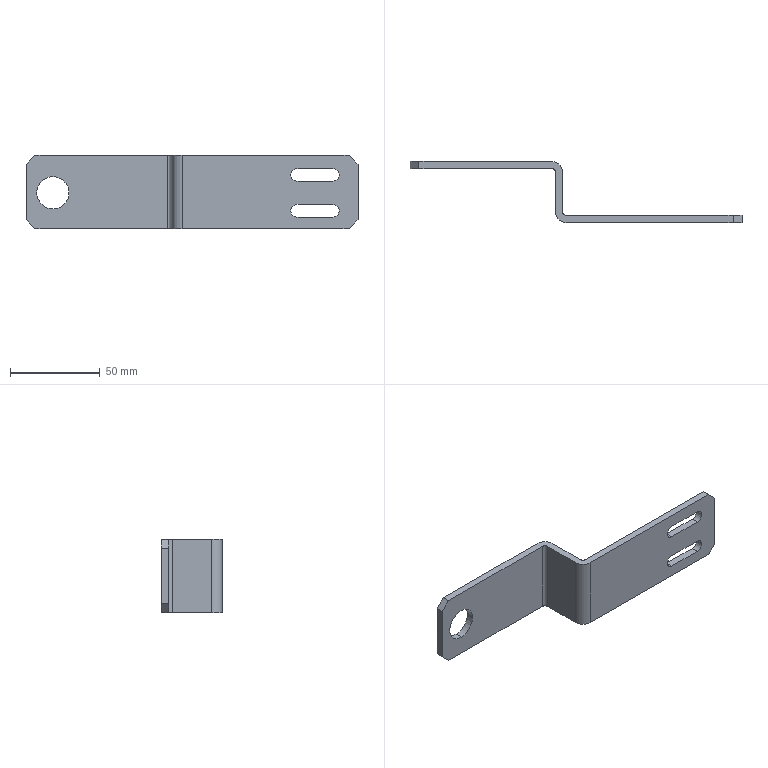Part | SolidWorks | features ICE 4, Fillet 2, Chamfer 1, Extrusion 1, HoleWzd 1 | 1 solid | 28 faces | box 185 x 34 x 40.884 mm | volume 31953 mm3 | plane 18 | cylinder 10 | commonest cylinder face diameters 7 x4 4 x2 12 x2 18 x2
STEP:
#1=CARTESIAN_POINT('',(15.,4.,29.));
#2=VERTEX_POINT('',#1);
#3=CARTESIAN_POINT('',(15.,4.,11.));
#4=VERTEX_POINT('',#3);
#5=CARTESIAN_POINT('',(15.,4.,20.));
#6=DIRECTION('',(0.,-1.,0.));
#7=DIRECTION('',(0.,0.,-1.));
#8=AXIS2_PLACEMENT_3D('',#5,#6,#7);
#9=CIRCLE('',#8,9.);
#10=EDGE_CURVE('',#2,#4,#9,.T.);
#11=ORIENTED_EDGE('',*,*,#10,.F.);
#12=CARTESIAN_POINT('',(15.,0.,29.));
#13=VERTEX_POINT('',#12);
#14=CARTESIAN_POINT('',(15.,0.,29.));
#15=DIRECTION('',(0.,-1.,0.));
#16=VECTOR('',#15,1000.);
#17=LINE('',#14,#16);
#18=EDGE_CURVE('',#2,#13,#17,.T.);
#19=ORIENTED_EDGE('',*,*,#18,.T.);
#20=CARTESIAN_POINT('',(15.,0.,11.));
#21=VERTEX_POINT('',#20);
#22=CARTESIAN_POINT('',(15.,0.,20.));
#23=DIRECTION('',(0.,-1.,0.));
#24=DIRECTION('',(0.,0.,-1.));
#25=AXIS2_PLACEMENT_3D('',#22,#23,#24);
#26=CIRCLE('',#25,9.);
#27=EDGE_CURVE('',#13,#21,#26,.T.);
#28=ORIENTED_EDGE('',*,*,#27,.T.);
#29=CARTESIAN_POINT('',(15.,0.,11.));
#30=DIRECTION('',(0.,-1.,0.));
#31=VECTOR('',#30,1000.);
#32=LINE('',#29,#31);
#33=EDGE_CURVE('',#4,#21,#32,.T.);
#34=ORIENTED_EDGE('',*,*,#33,.F.);
#35=EDGE_LOOP('',(#11,#19,#28,#34));
#36=FACE_OUTER_BOUND('',#35,.T.);
#37=CARTESIAN_POINT('',(15.,0.,20.));
#38=DIRECTION('',(0.,-1.,0.));
#39=DIRECTION('',(0.,0.,-1.));
#40=AXIS2_PLACEMENT_3D('',#37,#38,#39);
#41=CYLINDRICAL_SURFACE('',#40,9.);
#42=ADVANCED_FACE('',(#36),#41,.F.);
#43=CARTESIAN_POINT('',(0.,0.,35.884));
#44=VERTEX_POINT('',#43);
#45=CARTESIAN_POINT('',(0.,0.,5.));
#46=VERTEX_POINT('',#45);
#47=CARTESIAN_POINT('',(0.,0.,40.884));
#48=DIRECTION('',(0.,0.,-1.));
#49=VECTOR('',#48,1000.);
#50=LINE('',#47,#49);
#51=EDGE_CURVE('',#44,#46,#50,.T.);
#52=ORIENTED_EDGE('',*,*,#51,.F.);
#53=CARTESIAN_POINT('',(0.,4.,35.884));
#54=VERTEX_POINT('',#53);
#55=CARTESIAN_POINT('',(0.,4.,35.884));
#56=DIRECTION('',(0.,1.,0.));
#57=VECTOR('',#56,1000.);
#58=LINE('',#55,#57);
#59=EDGE_CURVE('',#44,#54,#58,.T.);
#60=ORIENTED_EDGE('',*,*,#59,.T.);
#61=CARTESIAN_POINT('',(0.,4.,5.));
#62=VERTEX_POINT('',#61);
#63=CARTESIAN_POINT('',(0.,4.,40.884));
#64=DIRECTION('',(0.,0.,-1.));
#65=VECTOR('',#64,1000.);
#66=LINE('',#63,#65);
#67=EDGE_CURVE('',#54,#62,#66,.T.);
#68=ORIENTED_EDGE('',*,*,#67,.T.);
#69=CARTESIAN_POINT('',(0.,4.,5.));
#70=DIRECTION('',(0.,-1.,0.));
#71=VECTOR('',#70,1000.);
#72=LINE('',#69,#71);
#73=EDGE_CURVE('',#62,#46,#72,.T.);
#74=ORIENTED_EDGE('',*,*,#73,.T.);
#75=EDGE_LOOP('',(#52,#60,#68,#74));
#76=FACE_OUTER_BOUND('',#75,.T.);
#77=CARTESIAN_POINT('',(0.,4.,40.884));
#78=DIRECTION('',(-1.,0.,0.));
#79=DIRECTION('',(0.,0.,1.));
#80=AXIS2_PLACEMENT_3D('',#77,#78,#79);
#81=PLANE('',#80);
#82=ADVANCED_FACE('',(#76),#81,.T.);
#83=CARTESIAN_POINT('',(81.,-2.,40.884));
#84=VERTEX_POINT('',#83);
#85=CARTESIAN_POINT('',(81.,-24.,40.884));
#86=VERTEX_POINT('',#85);
#87=CARTESIAN_POINT('',(81.,0.,40.884));
#88=DIRECTION('',(0.,-1.,0.));
#89=VECTOR('',#88,1000.);
#90=LINE('',#87,#89);
#91=EDGE_CURVE('',#84,#86,#90,.T.);
#92=ORIENTED_EDGE('',*,*,#91,.T.);
#93=CARTESIAN_POINT('',(87.,-30.,40.884));
#94=VERTEX_POINT('',#93);
#95=CARTESIAN_POINT('',(87.,-24.,40.884));
#96=DIRECTION('',(0.,0.,1.));
#97=DIRECTION('',(1.,0.,0.));
#98=AXIS2_PLACEMENT_3D('',#95,#96,#97);
#99=CIRCLE('',#98,6.);
#100=EDGE_CURVE('',#86,#94,#99,.T.);
#101=ORIENTED_EDGE('',*,*,#100,.T.);
#102=CARTESIAN_POINT('',(180.,-30.,40.884));
#103=VERTEX_POINT('',#102);
#104=CARTESIAN_POINT('',(185.,-30.,40.884));
#105=DIRECTION('',(-1.,0.,0.));
#106=VECTOR('',#105,1000.);
#107=LINE('',#104,#106);
#108=EDGE_CURVE('',#103,#94,#107,.T.);
#109=ORIENTED_EDGE('',*,*,#108,.F.);
#110=CARTESIAN_POINT('',(180.,-26.,40.884));
#111=VERTEX_POINT('',#110);
#112=CARTESIAN_POINT('',(180.,4.,40.884));
#113=DIRECTION('',(0.,1.,0.));
#114=VECTOR('',#113,1000.);
#115=LINE('',#112,#114);
#116=EDGE_CURVE('',#103,#111,#115,.T.);
#117=ORIENTED_EDGE('',*,*,#116,.T.);
#118=CARTESIAN_POINT('',(87.,-26.,40.884));
#119=VERTEX_POINT('',#118);
#120=CARTESIAN_POINT('',(185.,-26.,40.884));
#121=DIRECTION('',(-1.,0.,0.));
#122=VECTOR('',#121,1000.);
#123=LINE('',#120,#122);
#124=EDGE_CURVE('',#111,#119,#123,.T.);
#125=ORIENTED_EDGE('',*,*,#124,.T.);
#126=CARTESIAN_POINT('',(85.,-24.,40.884));
#127=VERTEX_POINT('',#126);
#128=CARTESIAN_POINT('',(87.,-24.,40.884));
#129=DIRECTION('',(0.,0.,-1.));
#130=DIRECTION('',(1.,0.,0.));
#131=AXIS2_PLACEMENT_3D('',#128,#129,#130);
#132=CIRCLE('',#131,2.);
#133=EDGE_CURVE('',#119,#127,#132,.T.);
#134=ORIENTED_EDGE('',*,*,#133,.T.);
#135=CARTESIAN_POINT('',(85.,-2.,40.884));
#136=VERTEX_POINT('',#135);
#137=CARTESIAN_POINT('',(85.,-26.,40.884));
#138=DIRECTION('',(0.,1.,0.));
#139=VECTOR('',#138,1000.);
#140=LINE('',#137,#139);
#141=EDGE_CURVE('',#127,#136,#140,.T.);
#142=ORIENTED_EDGE('',*,*,#141,.T.);
#143=CARTESIAN_POINT('',(79.,4.,40.884));
#144=VERTEX_POINT('',#143);
#145=CARTESIAN_POINT('',(79.,-2.,40.884));
#146=DIRECTION('',(0.,0.,1.));
#147=DIRECTION('',(1.,0.,0.));
#148=AXIS2_PLACEMENT_3D('',#145,#146,#147);
#149=CIRCLE('',#148,6.);
#150=EDGE_CURVE('',#136,#144,#149,.T.);
#151=ORIENTED_EDGE('',*,*,#150,.T.);
#152=CARTESIAN_POINT('',(5.,4.,40.884));
#153=VERTEX_POINT('',#152);
#154=CARTESIAN_POINT('',(185.,4.,40.884));
#155=DIRECTION('',(-1.,0.,0.));
#156=VECTOR('',#155,1000.);
#157=LINE('',#154,#156);
#158=EDGE_CURVE('',#144,#153,#157,.T.);
#159=ORIENTED_EDGE('',*,*,#158,.T.);
#160=CARTESIAN_POINT('',(5.,0.,40.884));
#161=VERTEX_POINT('',#160);
#162=CARTESIAN_POINT('',(5.,4.,40.884));
#163=DIRECTION('',(0.,-1.,0.));
#164=VECTOR('',#163,1000.);
#165=LINE('',#162,#164);
#166=EDGE_CURVE('',#153,#161,#165,.T.);
#167=ORIENTED_EDGE('',*,*,#166,.T.);
#168=CARTESIAN_POINT('',(79.,0.,40.884));
#169=VERTEX_POINT('',#168);
#170=CARTESIAN_POINT('',(0.,0.,40.884));
#171=DIRECTION('',(1.,0.,0.));
#172=VECTOR('',#171,1000.);
#173=LINE('',#170,#172);
#174=EDGE_CURVE('',#161,#169,#173,.T.);
#175=ORIENTED_EDGE('',*,*,#174,.T.);
#176=CARTESIAN_POINT('',(79.,-2.,40.884));
#177=DIRECTION('',(0.,0.,-1.));
#178=DIRECTION('',(1.,0.,0.));
#179=AXIS2_PLACEMENT_3D('',#176,#177,#178);
#180=CIRCLE('',#179,2.);
#181=EDGE_CURVE('',#169,#84,#180,.T.);
#182=ORIENTED_EDGE('',*,*,#181,.T.);
#183=EDGE_LOOP('',(#92,#101,#109,#117,#125,#134,#142,#151,#159,#167,#175,#182));
#184=FACE_OUTER_BOUND('',#183,.T.);
#185=CARTESIAN_POINT('',(185.,4.,40.884));
#186=DIRECTION('',(0.,0.,1.));
#187=DIRECTION('',(1.,0.,0.));
#188=AXIS2_PLACEMENT_3D('',#185,#186,#187);
#189=PLANE('',#188);
#190=ADVANCED_FACE('',(#184),#189,.T.);
#191=CARTESIAN_POINT('',(185.,-30.,5.));
#192=VERTEX_POINT('',#191);
#193=CARTESIAN_POINT('',(185.,-30.,35.884));
#194=VERTEX_POINT('',#193);
#195=CARTESIAN_POINT('',(185.,-30.,0.));
#196=DIRECTION('',(0.,0.,1.));
#197=VECTOR('',#196,1000.);
#198=LINE('',#195,#197);
#199=EDGE_CURVE('',#192,#194,#198,.T.);
#200=ORIENTED_EDGE('',*,*,#199,.F.);
#201=CARTESIAN_POINT('',(185.,-26.,5.));
#202=VERTEX_POINT('',#201);
#203=CARTESIAN_POINT('',(185.,4.,5.));
#204=DIRECTION('',(0.,1.,0.));
#205=VECTOR('',#204,1000.);
#206=LINE('',#203,#205);
#207=EDGE_CURVE('',#192,#202,#206,.T.);
#208=ORIENTED_EDGE('',*,*,#207,.T.);
#209=CARTESIAN_POINT('',(185.,-26.,35.884));
#210=VERTEX_POINT('',#209);
#211=CARTESIAN_POINT('',(185.,-26.,40.884));
#212=DIRECTION('',(0.,0.,-1.));
#213=VECTOR('',#212,1000.);
#214=LINE('',#211,#213);
#215=EDGE_CURVE('',#210,#202,#214,.T.);
#216=ORIENTED_EDGE('',*,*,#215,.F.);
#217=CARTESIAN_POINT('',(185.,4.,35.884));
#218=DIRECTION('',(0.,-1.,0.));
#219=VECTOR('',#218,1000.);
#220=LINE('',#217,#219);
#221=EDGE_CURVE('',#210,#194,#220,.T.);
#222=ORIENTED_EDGE('',*,*,#221,.T.);
#223=EDGE_LOOP('',(#200,#208,#216,#222));
#224=FACE_OUTER_BOUND('',#223,.T.);
#225=CARTESIAN_POINT('',(185.,4.,0.));
#226=DIRECTION('',(1.,0.,0.));
#227=DIRECTION('',(0.,0.,-1.));
#228=AXIS2_PLACEMENT_3D('',#225,#226,#227);
#229=PLANE('',#228);
#230=ADVANCED_FACE('',(#224),#229,.T.);
#231=CARTESIAN_POINT('',(87.,-30.,0.));
#232=VERTEX_POINT('',#231);
#233=CARTESIAN_POINT('',(180.,-30.,0.));
#234=VERTEX_POINT('',#233);
#235=CARTESIAN_POINT('',(0.,-30.,0.));
#236=DIRECTION('',(1.,0.,0.));
#237=VECTOR('',#236,1000.);
#238=LINE('',#235,#237);
#239=EDGE_CURVE('',#232,#234,#238,.T.);
#240=ORIENTED_EDGE('',*,*,#239,.F.);
#241=CARTESIAN_POINT('',(81.,-24.,0.));
#242=VERTEX_POINT('',#241);
#243=CARTESIAN_POINT('',(87.,-24.,0.));
#244=DIRECTION('',(0.,0.,-1.));
#245=DIRECTION('',(-1.,0.,0.));
#246=AXIS2_PLACEMENT_3D('',#243,#244,#245);
#247=CIRCLE('',#246,6.);
#248=EDGE_CURVE('',#232,#242,#247,.T.);
#249=ORIENTED_EDGE('',*,*,#248,.T.);
#250=CARTESIAN_POINT('',(81.,-2.,0.));
#251=VERTEX_POINT('',#250);
#252=CARTESIAN_POINT('',(81.,0.,0.));
#253=DIRECTION('',(0.,-1.,0.));
#254=VECTOR('',#253,1000.);
#255=LINE('',#252,#254);
#256=EDGE_CURVE('',#251,#242,#255,.T.);
#257=ORIENTED_EDGE('',*,*,#256,.F.);
#258=CARTESIAN_POINT('',(79.,0.,0.));
#259=VERTEX_POINT('',#258);
#260=CARTESIAN_POINT('',(79.,-2.,0.));
#261=DIRECTION('',(0.,0.,1.));
#262=DIRECTION('',(-1.,0.,0.));
#263=AXIS2_PLACEMENT_3D('',#260,#261,#262);
#264=CIRCLE('',#263,2.);
#265=EDGE_CURVE('',#251,#259,#264,.T.);
#266=ORIENTED_EDGE('',*,*,#265,.T.);
#267=CARTESIAN_POINT('',(5.,0.,0.));
#268=VERTEX_POINT('',#267);
#269=CARTESIAN_POINT('',(0.,0.,0.));
#270=DIRECTION('',(1.,0.,0.));
#271=VECTOR('',#270,1000.);
#272=LINE('',#269,#271);
#273=EDGE_CURVE('',#268,#259,#272,.T.);
#274=ORIENTED_EDGE('',*,*,#273,.F.);
#275=CARTESIAN_POINT('',(5.,4.,0.));
#276=VERTEX_POINT('',#275);
#277=CARTESIAN_POINT('',(5.,4.,0.));
#278=DIRECTION('',(0.,1.,0.));
#279=VECTOR('',#278,1000.);
#280=LINE('',#277,#279);
#281=EDGE_CURVE('',#268,#276,#280,.T.);
#282=ORIENTED_EDGE('',*,*,#281,.T.);
#283=CARTESIAN_POINT('',(79.,4.,0.));
#284=VERTEX_POINT('',#283);
#285=CARTESIAN_POINT('',(0.,4.,0.));
#286=DIRECTION('',(1.,0.,0.));
#287=VECTOR('',#286,1000.);
#288=LINE('',#285,#287);
#289=EDGE_CURVE('',#276,#284,#288,.T.);
#290=ORIENTED_EDGE('',*,*,#289,.T.);
#291=CARTESIAN_POINT('',(85.,-2.,0.));
#292=VERTEX_POINT('',#291);
#293=CARTESIAN_POINT('',(79.,-2.,0.));
#294=DIRECTION('',(0.,0.,-1.));
#295=DIRECTION('',(-1.,0.,0.));
#296=AXIS2_PLACEMENT_3D('',#293,#294,#295);
#297=CIRCLE('',#296,6.);
#298=EDGE_CURVE('',#284,#292,#297,.T.);
#299=ORIENTED_EDGE('',*,*,#298,.T.);
#300=CARTESIAN_POINT('',(85.,-24.,0.));
#301=VERTEX_POINT('',#300);
#302=CARTESIAN_POINT('',(85.,-26.,0.));
#303=DIRECTION('',(0.,1.,0.));
#304=VECTOR('',#303,1000.);
#305=LINE('',#302,#304);
#306=EDGE_CURVE('',#301,#292,#305,.T.);
#307=ORIENTED_EDGE('',*,*,#306,.F.);
#308=CARTESIAN_POINT('',(87.,-26.,0.));
#309=VERTEX_POINT('',#308);
#310=CARTESIAN_POINT('',(87.,-24.,0.));
#311=DIRECTION('',(0.,0.,1.));
#312=DIRECTION('',(-1.,0.,0.));
#313=AXIS2_PLACEMENT_3D('',#310,#311,#312);
#314=CIRCLE('',#313,2.);
#315=EDGE_CURVE('',#301,#309,#314,.T.);
#316=ORIENTED_EDGE('',*,*,#315,.T.);
#317=CARTESIAN_POINT('',(180.,-26.,0.));
#318=VERTEX_POINT('',#317);
#319=CARTESIAN_POINT('',(185.,-26.,0.));
#320=DIRECTION('',(-1.,0.,0.));
#321=VECTOR('',#320,1000.);
#322=LINE('',#319,#321);
#323=EDGE_CURVE('',#318,#309,#322,.T.);
#324=ORIENTED_EDGE('',*,*,#323,.F.);
#325=CARTESIAN_POINT('',(180.,4.,0.));
#326=DIRECTION('',(0.,-1.,0.));
#327=VECTOR('',#326,1000.);
#328=LINE('',#325,#327);
#329=EDGE_CURVE('',#318,#234,#328,.T.);
#330=ORIENTED_EDGE('',*,*,#329,.T.);
#331=EDGE_LOOP('',(#240,#249,#257,#266,#274,#282,#290,#299,#307,#316,#324,#330));
#332=FACE_OUTER_BOUND('',#331,.T.);
#333=CARTESIAN_POINT('',(0.,4.,0.));
#334=DIRECTION('',(0.,0.,-1.));
#335=DIRECTION('',(-1.,0.,0.));
#336=AXIS2_PLACEMENT_3D('',#333,#334,#335);
#337=PLANE('',#336);
#338=ADVANCED_FACE('',(#332),#337,.T.);
#339=CARTESIAN_POINT('',(15.,4.,20.));
#340=DIRECTION('',(0.,-1.,0.));
#341=DIRECTION('',(0.,0.,-1.));
#342=AXIS2_PLACEMENT_3D('',#339,#340,#341);
#343=CIRCLE('',#342,9.);
#344=EDGE_CURVE('',#4,#2,#343,.T.);
#345=ORIENTED_EDGE('',*,*,#344,.T.);
#346=ORIENTED_EDGE('',*,*,#10,.T.);
#347=EDGE_LOOP('',(#345,#346));
#348=FACE_BOUND('',#347,.T.);
#349=ORIENTED_EDGE('',*,*,#158,.F.);
#350=CARTESIAN_POINT('',(79.,4.,0.));
#351=DIRECTION('',(0.,0.,-1.));
#352=VECTOR('',#351,1000.);
#353=LINE('',#350,#352);
#354=EDGE_CURVE('',#144,#284,#353,.T.);
#355=ORIENTED_EDGE('',*,*,#354,.T.);
#356=ORIENTED_EDGE('',*,*,#289,.F.);
#357=CARTESIAN_POINT('',(0.,4.,5.));
#358=DIRECTION('',(-0.7071,0.,0.7071));
#359=VECTOR('',#358,1000.);
#360=LINE('',#357,#359);
#361=EDGE_CURVE('',#276,#62,#360,.T.);
#362=ORIENTED_EDGE('',*,*,#361,.T.);
#363=ORIENTED_EDGE('',*,*,#67,.F.);
#364=CARTESIAN_POINT('',(5.,4.,40.884));
#365=DIRECTION('',(0.7071,0.,0.7071));
#366=VECTOR('',#365,1000.);
#367=LINE('',#364,#366);
#368=EDGE_CURVE('',#54,#153,#367,.T.);
#369=ORIENTED_EDGE('',*,*,#368,.T.);
#370=EDGE_LOOP('',(#349,#355,#356,#362,#363,#369));
#371=FACE_OUTER_BOUND('',#370,.T.);
#372=CARTESIAN_POINT('',(0.,4.,0.));
#373=DIRECTION('',(0.,-1.,0.));
#374=DIRECTION('',(0.,0.,-1.));
#375=AXIS2_PLACEMENT_3D('',#372,#373,#374);
#376=PLANE('',#375);
#377=ADVANCED_FACE('',(#348,#371),#376,.F.);
#378=CARTESIAN_POINT('',(151.,-30.,26.5));
#379=VERTEX_POINT('',#378);
#380=CARTESIAN_POINT('',(151.,-30.,33.5));
#381=VERTEX_POINT('',#380);
#382=CARTESIAN_POINT('',(151.,-30.,30.));
#383=DIRECTION('',(0.,1.,0.));
#384=DIRECTION('',(0.,0.,1.));
#385=AXIS2_PLACEMENT_3D('',#382,#383,#384);
#386=CIRCLE('',#385,3.5);
#387=EDGE_CURVE('',#379,#381,#386,.T.);
#388=ORIENTED_EDGE('',*,*,#387,.T.);
#389=CARTESIAN_POINT('',(171.,-30.,33.5));
#390=VERTEX_POINT('',#389);
#391=CARTESIAN_POINT('',(151.,-30.,33.5));
#392=DIRECTION('',(1.,0.,0.));
#393=VECTOR('',#392,1000.);
#394=LINE('',#391,#393);
#395=EDGE_CURVE('',#381,#390,#394,.T.);
#396=ORIENTED_EDGE('',*,*,#395,.T.);
#397=CARTESIAN_POINT('',(171.,-30.,26.5));
#398=VERTEX_POINT('',#397);
#399=CARTESIAN_POINT('',(171.,-30.,30.));
#400=DIRECTION('',(0.,1.,0.));
#401=DIRECTION('',(0.,0.,1.));
#402=AXIS2_PLACEMENT_3D('',#399,#400,#401);
#403=CIRCLE('',#402,3.5);
#404=EDGE_CURVE('',#390,#398,#403,.T.);
#405=ORIENTED_EDGE('',*,*,#404,.T.);
#406=CARTESIAN_POINT('',(171.,-30.,26.5));
#407=DIRECTION('',(-1.,0.,0.));
#408=VECTOR('',#407,1000.);
#409=LINE('',#406,#408);
#410=EDGE_CURVE('',#398,#379,#409,.T.);
#411=ORIENTED_EDGE('',*,*,#410,.T.);
#412=EDGE_LOOP('',(#388,#396,#405,#411));
#413=FACE_BOUND('',#412,.T.);
#414=CARTESIAN_POINT('',(171.,-30.,6.5));
#415=VERTEX_POINT('',#414);
#416=CARTESIAN_POINT('',(171.,-30.,13.5));
#417=VERTEX_POINT('',#416);
#418=CARTESIAN_POINT('',(171.,-30.,10.));
#419=DIRECTION('',(0.,-1.,0.));
#420=DIRECTION('',(0.,0.,-1.));
#421=AXIS2_PLACEMENT_3D('',#418,#419,#420);
#422=CIRCLE('',#421,3.5);
#423=EDGE_CURVE('',#415,#417,#422,.T.);
#424=ORIENTED_EDGE('',*,*,#423,.F.);
#425=CARTESIAN_POINT('',(151.,-30.,6.5));
#426=VERTEX_POINT('',#425);
#427=CARTESIAN_POINT('',(151.,-30.,6.5));
#428=DIRECTION('',(1.,0.,0.));
#429=VECTOR('',#428,1000.);
#430=LINE('',#427,#429);
#431=EDGE_CURVE('',#426,#415,#430,.T.);
#432=ORIENTED_EDGE('',*,*,#431,.F.);
#433=CARTESIAN_POINT('',(151.,-30.,13.5));
#434=VERTEX_POINT('',#433);
#435=CARTESIAN_POINT('',(151.,-30.,10.));
#436=DIRECTION('',(0.,-1.,0.));
#437=DIRECTION('',(0.,0.,-1.));
#438=AXIS2_PLACEMENT_3D('',#435,#436,#437);
#439=CIRCLE('',#438,3.5);
#440=EDGE_CURVE('',#434,#426,#439,.T.);
#441=ORIENTED_EDGE('',*,*,#440,.F.);
#442=CARTESIAN_POINT('',(171.,-30.,13.5));
#443=DIRECTION('',(-1.,0.,0.));
#444=VECTOR('',#443,1000.);
#445=LINE('',#442,#444);
#446=EDGE_CURVE('',#417,#434,#445,.T.);
#447=ORIENTED_EDGE('',*,*,#446,.F.);
#448=EDGE_LOOP('',(#424,#432,#441,#447));
#449=FACE_BOUND('',#448,.T.);
#450=ORIENTED_EDGE('',*,*,#108,.T.);
#451=CARTESIAN_POINT('',(87.,-30.,0.));
#452=DIRECTION('',(0.,0.,-1.));
#453=VECTOR('',#452,1000.);
#454=LINE('',#451,#453);
#455=EDGE_CURVE('',#94,#232,#454,.T.);
#456=ORIENTED_EDGE('',*,*,#455,.T.);
#457=ORIENTED_EDGE('',*,*,#239,.T.);
#458=CARTESIAN_POINT('',(90.,-30.,-90.));
#459=DIRECTION('',(0.7071,0.,0.7071));
#460=VECTOR('',#459,1000.);
#461=LINE('',#458,#460);
#462=EDGE_CURVE('',#234,#192,#461,.T.);
#463=ORIENTED_EDGE('',*,*,#462,.T.);
#464=ORIENTED_EDGE('',*,*,#199,.T.);
#465=CARTESIAN_POINT('',(110.442,-30.,110.442));
#466=DIRECTION('',(-0.7071,0.,0.7071));
#467=VECTOR('',#466,1000.);
#468=LINE('',#465,#467);
#469=EDGE_CURVE('',#194,#103,#468,.T.);
#470=ORIENTED_EDGE('',*,*,#469,.T.);
#471=EDGE_LOOP('',(#450,#456,#457,#463,#464,#470));
#472=FACE_OUTER_BOUND('',#471,.T.);
#473=CARTESIAN_POINT('',(0.,-30.,0.));
#474=DIRECTION('',(0.,-1.,0.));
#475=DIRECTION('',(0.,0.,-1.));
#476=AXIS2_PLACEMENT_3D('',#473,#474,#475);
#477=PLANE('',#476);
#478=ADVANCED_FACE('',(#413,#449,#472),#477,.T.);
#479=ORIENTED_EDGE('',*,*,#306,.T.);
#480=CARTESIAN_POINT('',(85.,-2.,40.884));
#481=DIRECTION('',(0.,0.,1.));
#482=VECTOR('',#481,1000.);
#483=LINE('',#480,#482);
#484=EDGE_CURVE('',#292,#136,#483,.T.);
#485=ORIENTED_EDGE('',*,*,#484,.T.);
#486=ORIENTED_EDGE('',*,*,#141,.F.);
#487=CARTESIAN_POINT('',(85.,-24.,0.));
#488=DIRECTION('',(0.,0.,-1.));
#489=VECTOR('',#488,1000.);
#490=LINE('',#487,#489);
#491=EDGE_CURVE('',#127,#301,#490,.T.);
#492=ORIENTED_EDGE('',*,*,#491,.T.);
#493=EDGE_LOOP('',(#479,#485,#486,#492));
#494=FACE_OUTER_BOUND('',#493,.T.);
#495=CARTESIAN_POINT('',(85.,-26.,40.884));
#496=DIRECTION('',(-1.,0.,0.));
#497=DIRECTION('',(0.,-1.,0.));
#498=AXIS2_PLACEMENT_3D('',#495,#496,#497);
#499=PLANE('',#498);
#500=ADVANCED_FACE('',(#494),#499,.F.);
#501=CARTESIAN_POINT('',(151.,-26.,33.5));
#502=VERTEX_POINT('',#501);
#503=CARTESIAN_POINT('',(171.,-26.,33.5));
#504=VERTEX_POINT('',#503);
#505=CARTESIAN_POINT('',(151.,-26.,33.5));
#506=DIRECTION('',(1.,0.,0.));
#507=VECTOR('',#506,1000.);
#508=LINE('',#505,#507);
#509=EDGE_CURVE('',#502,#504,#508,.T.);
#510=ORIENTED_EDGE('',*,*,#509,.F.);
#511=CARTESIAN_POINT('',(151.,-26.,26.5));
#512=VERTEX_POINT('',#511);
#513=CARTESIAN_POINT('',(151.,-26.,30.));
#514=DIRECTION('',(0.,1.,0.));
#515=DIRECTION('',(0.,0.,1.));
#516=AXIS2_PLACEMENT_3D('',#513,#514,#515);
#517=CIRCLE('',#516,3.5);
#518=EDGE_CURVE('',#512,#502,#517,.T.);
#519=ORIENTED_EDGE('',*,*,#518,.F.);
#520=CARTESIAN_POINT('',(171.,-26.,26.5));
#521=VERTEX_POINT('',#520);
#522=CARTESIAN_POINT('',(171.,-26.,26.5));
#523=DIRECTION('',(-1.,0.,0.));
#524=VECTOR('',#523,1000.);
#525=LINE('',#522,#524);
#526=EDGE_CURVE('',#521,#512,#525,.T.);
#527=ORIENTED_EDGE('',*,*,#526,.F.);
#528=CARTESIAN_POINT('',(171.,-26.,30.));
#529=DIRECTION('',(0.,1.,0.));
#530=DIRECTION('',(0.,0.,1.));
#531=AXIS2_PLACEMENT_3D('',#528,#529,#530);
#532=CIRCLE('',#531,3.5);
#533=EDGE_CURVE('',#504,#521,#532,.T.);
#534=ORIENTED_EDGE('',*,*,#533,.F.);
#535=EDGE_LOOP('',(#510,#519,#527,#534));
#536=FACE_BOUND('',#535,.T.);
#537=CARTESIAN_POINT('',(151.,-26.,6.5));
#538=VERTEX_POINT('',#537);
#539=CARTESIAN_POINT('',(171.,-26.,6.5));
#540=VERTEX_POINT('',#539);
#541=CARTESIAN_POINT('',(185.,-26.,6.5));
#542=DIRECTION('',(1.,0.,0.));
#543=VECTOR('',#542,1000.);
#544=LINE('',#541,#543);
#545=EDGE_CURVE('',#538,#540,#544,.T.);
#546=ORIENTED_EDGE('',*,*,#545,.T.);
#547=CARTESIAN_POINT('',(171.,-26.,13.5));
#548=VERTEX_POINT('',#547);
#549=CARTESIAN_POINT('',(171.,-26.,10.));
#550=DIRECTION('',(0.,-1.,0.));
#551=DIRECTION('',(0.,0.,-1.));
#552=AXIS2_PLACEMENT_3D('',#549,#550,#551);
#553=CIRCLE('',#552,3.5);
#554=EDGE_CURVE('',#540,#548,#553,.T.);
#555=ORIENTED_EDGE('',*,*,#554,.T.);
#556=CARTESIAN_POINT('',(151.,-26.,13.5));
#557=VERTEX_POINT('',#556);
#558=CARTESIAN_POINT('',(185.,-26.,13.5));
#559=DIRECTION('',(-1.,0.,0.));
#560=VECTOR('',#559,1000.);
#561=LINE('',#558,#560);
#562=EDGE_CURVE('',#548,#557,#561,.T.);
#563=ORIENTED_EDGE('',*,*,#562,.T.);
#564=CARTESIAN_POINT('',(151.,-26.,10.));
#565=DIRECTION('',(0.,-1.,0.));
#566=DIRECTION('',(0.,0.,-1.));
#567=AXIS2_PLACEMENT_3D('',#564,#565,#566);
#568=CIRCLE('',#567,3.5);
#569=EDGE_CURVE('',#557,#538,#568,.T.);
#570=ORIENTED_EDGE('',*,*,#569,.T.);
#571=EDGE_LOOP('',(#546,#555,#563,#570));
#572=FACE_BOUND('',#571,.T.);
#573=ORIENTED_EDGE('',*,*,#323,.T.);
#574=CARTESIAN_POINT('',(87.,-26.,40.884));
#575=DIRECTION('',(0.,0.,1.));
#576=VECTOR('',#575,1000.);
#577=LINE('',#574,#576);
#578=EDGE_CURVE('',#309,#119,#577,.T.);
#579=ORIENTED_EDGE('',*,*,#578,.T.);
#580=ORIENTED_EDGE('',*,*,#124,.F.);
#581=CARTESIAN_POINT('',(185.,-26.,35.884));
#582=DIRECTION('',(0.7071,0.,-0.7071));
#583=VECTOR('',#582,1000.);
#584=LINE('',#581,#583);
#585=EDGE_CURVE('',#111,#210,#584,.T.);
#586=ORIENTED_EDGE('',*,*,#585,.T.);
#587=ORIENTED_EDGE('',*,*,#215,.T.);
#588=CARTESIAN_POINT('',(180.,-26.,0.));
#589=DIRECTION('',(-0.7071,0.,-0.7071));
#590=VECTOR('',#589,1000.);
#591=LINE('',#588,#590);
#592=EDGE_CURVE('',#202,#318,#591,.T.);
#593=ORIENTED_EDGE('',*,*,#592,.T.);
#594=EDGE_LOOP('',(#573,#579,#580,#586,#587,#593));
#595=FACE_OUTER_BOUND('',#594,.T.);
#596=CARTESIAN_POINT('',(185.,-26.,40.884));
#597=DIRECTION('',(0.,-1.,0.));
#598=DIRECTION('',(0.,0.,-1.));
#599=AXIS2_PLACEMENT_3D('',#596,#597,#598);
#600=PLANE('',#599);
#601=ADVANCED_FACE('',(#536,#572,#595),#600,.F.);
#602=ORIENTED_EDGE('',*,*,#256,.T.);
#603=CARTESIAN_POINT('',(81.,-24.,40.884));
#604=DIRECTION('',(0.,0.,1.));
#605=VECTOR('',#604,1000.);
#606=LINE('',#603,#605);
#607=EDGE_CURVE('',#242,#86,#606,.T.);
#608=ORIENTED_EDGE('',*,*,#607,.T.);
#609=ORIENTED_EDGE('',*,*,#91,.F.);
#610=CARTESIAN_POINT('',(81.,-2.,0.));
#611=DIRECTION('',(0.,0.,-1.));
#612=VECTOR('',#611,1000.);
#613=LINE('',#610,#612);
#614=EDGE_CURVE('',#84,#251,#613,.T.);
#615=ORIENTED_EDGE('',*,*,#614,.T.);
#616=EDGE_LOOP('',(#602,#608,#609,#615));
#617=FACE_OUTER_BOUND('',#616,.T.);
#618=CARTESIAN_POINT('',(81.,0.,40.884));
#619=DIRECTION('',(1.,0.,0.));
#620=DIRECTION('',(0.,0.,-1.));
#621=AXIS2_PLACEMENT_3D('',#618,#619,#620);
#622=PLANE('',#621);
#623=ADVANCED_FACE('',(#617),#622,.F.);
#624=CARTESIAN_POINT('',(15.,0.,20.));
#625=DIRECTION('',(0.,-1.,0.));
#626=DIRECTION('',(0.,0.,-1.));
#627=AXIS2_PLACEMENT_3D('',#624,#625,#626);
#628=CIRCLE('',#627,9.);
#629=EDGE_CURVE('',#21,#13,#628,.T.);
#630=ORIENTED_EDGE('',*,*,#629,.F.);
#631=ORIENTED_EDGE('',*,*,#27,.F.);
#632=EDGE_LOOP('',(#630,#631));
#633=FACE_BOUND('',#632,.T.);
#634=ORIENTED_EDGE('',*,*,#273,.T.);
#635=CARTESIAN_POINT('',(79.,0.,40.884));
#636=DIRECTION('',(0.,0.,1.));
#637=VECTOR('',#636,1000.);
#638=LINE('',#635,#637);
#639=EDGE_CURVE('',#259,#169,#638,.T.);
#640=ORIENTED_EDGE('',*,*,#639,.T.);
#641=ORIENTED_EDGE('',*,*,#174,.F.);
#642=CARTESIAN_POINT('',(5.,0.,40.884));
#643=DIRECTION('',(-0.7071,0.,-0.7071));
#644=VECTOR('',#643,1000.);
#645=LINE('',#642,#644);
#646=EDGE_CURVE('',#161,#44,#645,.T.);
#647=ORIENTED_EDGE('',*,*,#646,.T.);
#648=ORIENTED_EDGE('',*,*,#51,.T.);
#649=CARTESIAN_POINT('',(0.,0.,5.));
#650=DIRECTION('',(0.7071,0.,-0.7071));
#651=VECTOR('',#650,1000.);
#652=LINE('',#649,#651);
#653=EDGE_CURVE('',#46,#268,#652,.T.);
#654=ORIENTED_EDGE('',*,*,#653,.T.);
#655=EDGE_LOOP('',(#634,#640,#641,#647,#648,#654));
#656=FACE_OUTER_BOUND('',#655,.T.);
#657=CARTESIAN_POINT('',(0.,0.,40.884));
#658=DIRECTION('',(0.,1.,0.));
#659=DIRECTION('',(-1.,0.,0.));
#660=AXIS2_PLACEMENT_3D('',#657,#658,#659);
#661=PLANE('',#660);
#662=ADVANCED_FACE('',(#633,#656),#661,.F.);
#663=CARTESIAN_POINT('',(171.,4.,6.5));
#664=DIRECTION('',(0.,-1.,0.));
#665=VECTOR('',#664,1000.);
#666=LINE('',#663,#665);
#667=EDGE_CURVE('',#540,#415,#666,.T.);
#668=ORIENTED_EDGE('',*,*,#667,.T.);
#669=ORIENTED_EDGE('',*,*,#423,.T.);
#670=CARTESIAN_POINT('',(171.,4.,13.5));
#671=DIRECTION('',(0.,-1.,0.));
#672=VECTOR('',#671,1000.);
#673=LINE('',#670,#672);
#674=EDGE_CURVE('',#548,#417,#673,.T.);
#675=ORIENTED_EDGE('',*,*,#674,.F.);
#676=ORIENTED_EDGE('',*,*,#554,.F.);
#677=EDGE_LOOP('',(#668,#669,#675,#676));
#678=FACE_OUTER_BOUND('',#677,.T.);
#679=CARTESIAN_POINT('',(171.,4.,10.));
#680=DIRECTION('',(0.,-1.,0.));
#681=DIRECTION('',(0.,0.,-1.));
#682=AXIS2_PLACEMENT_3D('',#679,#680,#681);
#683=CYLINDRICAL_SURFACE('',#682,3.5);
#684=ADVANCED_FACE('',(#678),#683,.F.);
#685=CARTESIAN_POINT('',(151.,4.,6.5));
#686=DIRECTION('',(0.,-1.,0.));
#687=VECTOR('',#686,1000.);
#688=LINE('',#685,#687);
#689=EDGE_CURVE('',#538,#426,#688,.T.);
#690=ORIENTED_EDGE('',*,*,#689,.T.);
#691=ORIENTED_EDGE('',*,*,#431,.T.);
#692=ORIENTED_EDGE('',*,*,#667,.F.);
#693=ORIENTED_EDGE('',*,*,#545,.F.);
#694=EDGE_LOOP('',(#690,#691,#692,#693));
#695=FACE_OUTER_BOUND('',#694,.T.);
#696=CARTESIAN_POINT('',(151.,4.,6.5));
#697=DIRECTION('',(0.,0.,-1.));
#698=DIRECTION('',(-1.,0.,0.));
#699=AXIS2_PLACEMENT_3D('',#696,#697,#698);
#700=PLANE('',#699);
#701=ADVANCED_FACE('',(#695),#700,.F.);
#702=CARTESIAN_POINT('',(151.,4.,13.5));
#703=DIRECTION('',(0.,-1.,0.));
#704=VECTOR('',#703,1000.);
#705=LINE('',#702,#704);
#706=EDGE_CURVE('',#557,#434,#705,.T.);
#707=ORIENTED_EDGE('',*,*,#706,.T.);
#708=ORIENTED_EDGE('',*,*,#440,.T.);
#709=ORIENTED_EDGE('',*,*,#689,.F.);
#710=ORIENTED_EDGE('',*,*,#569,.F.);
#711=EDGE_LOOP('',(#707,#708,#709,#710));
#712=FACE_OUTER_BOUND('',#711,.T.);
#713=CARTESIAN_POINT('',(151.,4.,10.));
#714=DIRECTION('',(0.,-1.,0.));
#715=DIRECTION('',(0.,0.,-1.));
#716=AXIS2_PLACEMENT_3D('',#713,#714,#715);
#717=CYLINDRICAL_SURFACE('',#716,3.5);
#718=ADVANCED_FACE('',(#712),#717,.F.);
#719=ORIENTED_EDGE('',*,*,#674,.T.);
#720=ORIENTED_EDGE('',*,*,#446,.T.);
#721=ORIENTED_EDGE('',*,*,#706,.F.);
#722=ORIENTED_EDGE('',*,*,#562,.F.);
#723=EDGE_LOOP('',(#719,#720,#721,#722));
#724=FACE_OUTER_BOUND('',#723,.T.);
#725=CARTESIAN_POINT('',(171.,4.,13.5));
#726=DIRECTION('',(0.,0.,1.));
#727=DIRECTION('',(1.,0.,0.));
#728=AXIS2_PLACEMENT_3D('',#725,#726,#727);
#729=PLANE('',#728);
#730=ADVANCED_FACE('',(#724),#729,.F.);
#731=ORIENTED_EDGE('',*,*,#518,.T.);
#732=CARTESIAN_POINT('',(151.,-30.,33.5));
#733=DIRECTION('',(0.,1.,0.));
#734=VECTOR('',#733,1000.);
#735=LINE('',#732,#734);
#736=EDGE_CURVE('',#381,#502,#735,.T.);
#737=ORIENTED_EDGE('',*,*,#736,.F.);
#738=ORIENTED_EDGE('',*,*,#387,.F.);
#739=CARTESIAN_POINT('',(151.,-30.,26.5));
#740=DIRECTION('',(0.,1.,0.));
#741=VECTOR('',#740,1000.);
#742=LINE('',#739,#741);
#743=EDGE_CURVE('',#379,#512,#742,.T.);
#744=ORIENTED_EDGE('',*,*,#743,.T.);
#745=EDGE_LOOP('',(#731,#737,#738,#744));
#746=FACE_OUTER_BOUND('',#745,.T.);
#747=CARTESIAN_POINT('',(151.,-30.,30.));
#748=DIRECTION('',(0.,1.,0.));
#749=DIRECTION('',(0.,0.,1.));
#750=AXIS2_PLACEMENT_3D('',#747,#748,#749);
#751=CYLINDRICAL_SURFACE('',#750,3.5);
#752=ADVANCED_FACE('',(#746),#751,.F.);
#753=ORIENTED_EDGE('',*,*,#526,.T.);
#754=ORIENTED_EDGE('',*,*,#743,.F.);
#755=ORIENTED_EDGE('',*,*,#410,.F.);
#756=CARTESIAN_POINT('',(171.,-30.,26.5));
#757=DIRECTION('',(0.,1.,0.));
#758=VECTOR('',#757,1000.);
#759=LINE('',#756,#758);
#760=EDGE_CURVE('',#398,#521,#759,.T.);
#761=ORIENTED_EDGE('',*,*,#760,.T.);
#762=EDGE_LOOP('',(#753,#754,#755,#761));
#763=FACE_OUTER_BOUND('',#762,.T.);
#764=CARTESIAN_POINT('',(171.,-30.,26.5));
#765=DIRECTION('',(0.,0.,-1.));
#766=DIRECTION('',(-1.,0.,0.));
#767=AXIS2_PLACEMENT_3D('',#764,#765,#766);
#768=PLANE('',#767);
#769=ADVANCED_FACE('',(#763),#768,.F.);
#770=ORIENTED_EDGE('',*,*,#533,.T.);
#771=ORIENTED_EDGE('',*,*,#760,.F.);
#772=ORIENTED_EDGE('',*,*,#404,.F.);
#773=CARTESIAN_POINT('',(171.,-30.,33.5));
#774=DIRECTION('',(0.,1.,0.));
#775=VECTOR('',#774,1000.);
#776=LINE('',#773,#775);
#777=EDGE_CURVE('',#390,#504,#776,.T.);
#778=ORIENTED_EDGE('',*,*,#777,.T.);
#779=EDGE_LOOP('',(#770,#771,#772,#778));
#780=FACE_OUTER_BOUND('',#779,.T.);
#781=CARTESIAN_POINT('',(171.,-30.,30.));
#782=DIRECTION('',(0.,1.,0.));
#783=DIRECTION('',(0.,0.,1.));
#784=AXIS2_PLACEMENT_3D('',#781,#782,#783);
#785=CYLINDRICAL_SURFACE('',#784,3.5);
#786=ADVANCED_FACE('',(#780),#785,.F.);
#787=ORIENTED_EDGE('',*,*,#509,.T.);
#788=ORIENTED_EDGE('',*,*,#777,.F.);
#789=ORIENTED_EDGE('',*,*,#395,.F.);
#790=ORIENTED_EDGE('',*,*,#736,.T.);
#791=EDGE_LOOP('',(#787,#788,#789,#790));
#792=FACE_OUTER_BOUND('',#791,.T.);
#793=CARTESIAN_POINT('',(151.,-30.,33.5));
#794=DIRECTION('',(0.,0.,1.));
#795=DIRECTION('',(1.,0.,0.));
#796=AXIS2_PLACEMENT_3D('',#793,#794,#795);
#797=PLANE('',#796);
#798=ADVANCED_FACE('',(#792),#797,.F.);
#799=ORIENTED_EDGE('',*,*,#18,.F.);
#800=ORIENTED_EDGE('',*,*,#344,.F.);
#801=ORIENTED_EDGE('',*,*,#33,.T.);
#802=ORIENTED_EDGE('',*,*,#629,.T.);
#803=EDGE_LOOP('',(#799,#800,#801,#802));
#804=FACE_OUTER_BOUND('',#803,.T.);
#805=CARTESIAN_POINT('',(15.,0.,20.));
#806=DIRECTION('',(0.,-1.,0.));
#807=DIRECTION('',(0.,0.,-1.));
#808=AXIS2_PLACEMENT_3D('',#805,#806,#807);
#809=CYLINDRICAL_SURFACE('',#808,9.);
#810=ADVANCED_FACE('',(#804),#809,.F.);
#811=ORIENTED_EDGE('',*,*,#368,.F.);
#812=ORIENTED_EDGE('',*,*,#59,.F.);
#813=ORIENTED_EDGE('',*,*,#646,.F.);
#814=ORIENTED_EDGE('',*,*,#166,.F.);
#815=EDGE_LOOP('',(#811,#812,#813,#814));
#816=FACE_OUTER_BOUND('',#815,.T.);
#817=CARTESIAN_POINT('',(5.,4.,40.884));
#818=DIRECTION('',(0.7071,0.,-0.7071));
#819=DIRECTION('',(0.,-1.,0.));
#820=AXIS2_PLACEMENT_3D('',#817,#818,#819);
#821=PLANE('',#820);
#822=ADVANCED_FACE('',(#816),#821,.F.);
#823=ORIENTED_EDGE('',*,*,#592,.F.);
#824=ORIENTED_EDGE('',*,*,#207,.F.);
#825=ORIENTED_EDGE('',*,*,#462,.F.);
#826=ORIENTED_EDGE('',*,*,#329,.F.);
#827=EDGE_LOOP('',(#823,#824,#825,#826));
#828=FACE_OUTER_BOUND('',#827,.T.);
#829=CARTESIAN_POINT('',(180.,4.,0.));
#830=DIRECTION('',(-0.7071,0.,0.7071));
#831=DIRECTION('',(0.,-1.,0.));
#832=AXIS2_PLACEMENT_3D('',#829,#830,#831);
#833=PLANE('',#832);
#834=ADVANCED_FACE('',(#828),#833,.F.);
#835=ORIENTED_EDGE('',*,*,#361,.F.);
#836=ORIENTED_EDGE('',*,*,#281,.F.);
#837=ORIENTED_EDGE('',*,*,#653,.F.);
#838=ORIENTED_EDGE('',*,*,#73,.F.);
#839=EDGE_LOOP('',(#835,#836,#837,#838));
#840=FACE_OUTER_BOUND('',#839,.T.);
#841=CARTESIAN_POINT('',(0.,4.,5.));
#842=DIRECTION('',(0.7071,0.,0.7071));
#843=DIRECTION('',(0.,-1.,0.));
#844=AXIS2_PLACEMENT_3D('',#841,#842,#843);
#845=PLANE('',#844);
#846=ADVANCED_FACE('',(#840),#845,.F.);
#847=ORIENTED_EDGE('',*,*,#585,.F.);
#848=ORIENTED_EDGE('',*,*,#116,.F.);
#849=ORIENTED_EDGE('',*,*,#469,.F.);
#850=ORIENTED_EDGE('',*,*,#221,.F.);
#851=EDGE_LOOP('',(#847,#848,#849,#850));
#852=FACE_OUTER_BOUND('',#851,.T.);
#853=CARTESIAN_POINT('',(185.,4.,35.884));
#854=DIRECTION('',(-0.7071,0.,-0.7071));
#855=DIRECTION('',(0.,-1.,0.));
#856=AXIS2_PLACEMENT_3D('',#853,#854,#855);
#857=PLANE('',#856);
#858=ADVANCED_FACE('',(#852),#857,.F.);
#859=ORIENTED_EDGE('',*,*,#133,.F.);
#860=ORIENTED_EDGE('',*,*,#578,.F.);
#861=ORIENTED_EDGE('',*,*,#315,.F.);
#862=ORIENTED_EDGE('',*,*,#491,.F.);
#863=EDGE_LOOP('',(#859,#860,#861,#862));
#864=FACE_OUTER_BOUND('',#863,.T.);
#865=CARTESIAN_POINT('',(87.,-24.,40.884));
#866=DIRECTION('',(0.,0.,1.));
#867=DIRECTION('',(1.,0.,0.));
#868=AXIS2_PLACEMENT_3D('',#865,#866,#867);
#869=CYLINDRICAL_SURFACE('',#868,2.);
#870=ADVANCED_FACE('',(#864),#869,.F.);
#871=ORIENTED_EDGE('',*,*,#181,.F.);
#872=ORIENTED_EDGE('',*,*,#639,.F.);
#873=ORIENTED_EDGE('',*,*,#265,.F.);
#874=ORIENTED_EDGE('',*,*,#614,.F.);
#875=EDGE_LOOP('',(#871,#872,#873,#874));
#876=FACE_OUTER_BOUND('',#875,.T.);
#877=CARTESIAN_POINT('',(79.,-2.,40.884));
#878=DIRECTION('',(0.,0.,1.));
#879=DIRECTION('',(1.,0.,0.));
#880=AXIS2_PLACEMENT_3D('',#877,#878,#879);
#881=CYLINDRICAL_SURFACE('',#880,2.);
#882=ADVANCED_FACE('',(#876),#881,.F.);
#883=ORIENTED_EDGE('',*,*,#100,.F.);
#884=ORIENTED_EDGE('',*,*,#607,.F.);
#885=ORIENTED_EDGE('',*,*,#248,.F.);
#886=ORIENTED_EDGE('',*,*,#455,.F.);
#887=EDGE_LOOP('',(#883,#884,#885,#886));
#888=FACE_OUTER_BOUND('',#887,.T.);
#889=CARTESIAN_POINT('',(87.,-24.,0.));
#890=DIRECTION('',(0.,0.,1.));
#891=DIRECTION('',(1.,0.,0.));
#892=AXIS2_PLACEMENT_3D('',#889,#890,#891);
#893=CYLINDRICAL_SURFACE('',#892,6.);
#894=ADVANCED_FACE('',(#888),#893,.T.);
#895=ORIENTED_EDGE('',*,*,#150,.F.);
#896=ORIENTED_EDGE('',*,*,#484,.F.);
#897=ORIENTED_EDGE('',*,*,#298,.F.);
#898=ORIENTED_EDGE('',*,*,#354,.F.);
#899=EDGE_LOOP('',(#895,#896,#897,#898));
#900=FACE_OUTER_BOUND('',#899,.T.);
#901=CARTESIAN_POINT('',(79.,-2.,0.));
#902=DIRECTION('',(0.,0.,-1.));
#903=DIRECTION('',(-1.,0.,0.));
#904=AXIS2_PLACEMENT_3D('',#901,#902,#903);
#905=CYLINDRICAL_SURFACE('',#904,6.);
#906=ADVANCED_FACE('',(#900),#905,.T.);
#907=CLOSED_SHELL('',(#42,#82,#190,#230,#338,#377,#478,#500,#601,#623,#662,#684,#701,#718,#730,#752,#769,#786,#798,#810,#822,#834,#846,#858,#870,#882,#894,#906));
#908=MANIFOLD_SOLID_BREP('',#907);
#909=CARTESIAN_POINT('',(0.,0.,0.));
#910=DIRECTION('',(0.,0.,1.));
#911=DIRECTION('',(1.,0.,0.));
#912=AXIS2_PLACEMENT_3D('',#909,#910,#911);
#913=(LENGTH_UNIT()NAMED_UNIT(*)SI_UNIT(.MILLI.,.METRE.));
#914=UNCERTAINTY_MEASURE_WITH_UNIT(LENGTH_MEASURE(0.00001),#913,'','');
#915=(NAMED_UNIT(*)PLANE_ANGLE_UNIT()SI_UNIT($,.RADIAN.));
#916=(NAMED_UNIT(*)SI_UNIT($,.STERADIAN.)SOLID_ANGLE_UNIT());
#917=(GEOMETRIC_REPRESENTATION_CONTEXT(3)GLOBAL_UNCERTAINTY_ASSIGNED_CONTEXT((#914))GLOBAL_UNIT_ASSIGNED_CONTEXT((#913,#915,#916))REPRESENTATION_CONTEXT('',''));
#918=ADVANCED_BREP_SHAPE_REPRESENTATION('',(#908,#912),#917);